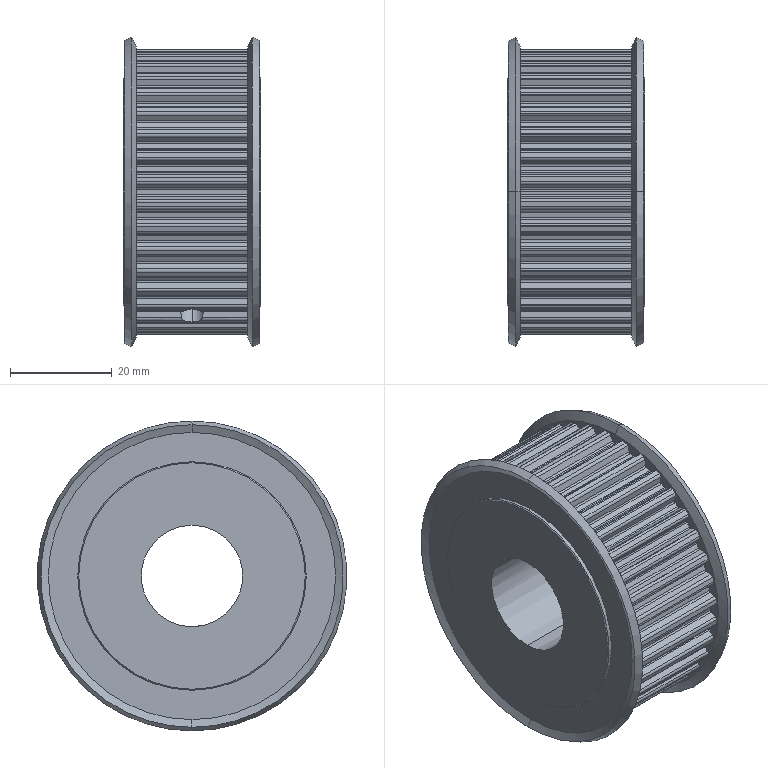Part | SolidWorks | features BaseBody 1 | 1 solid | 362 faces | box 27 x 61 x 61 mm | volume 54689 mm3 | cylinder 266 | plane 82 | cone 14 | commonest cylinder face diameters 0.8 x91 1.2 x90 52.85 x39 56.45 x36 4.917 x4 45 x4